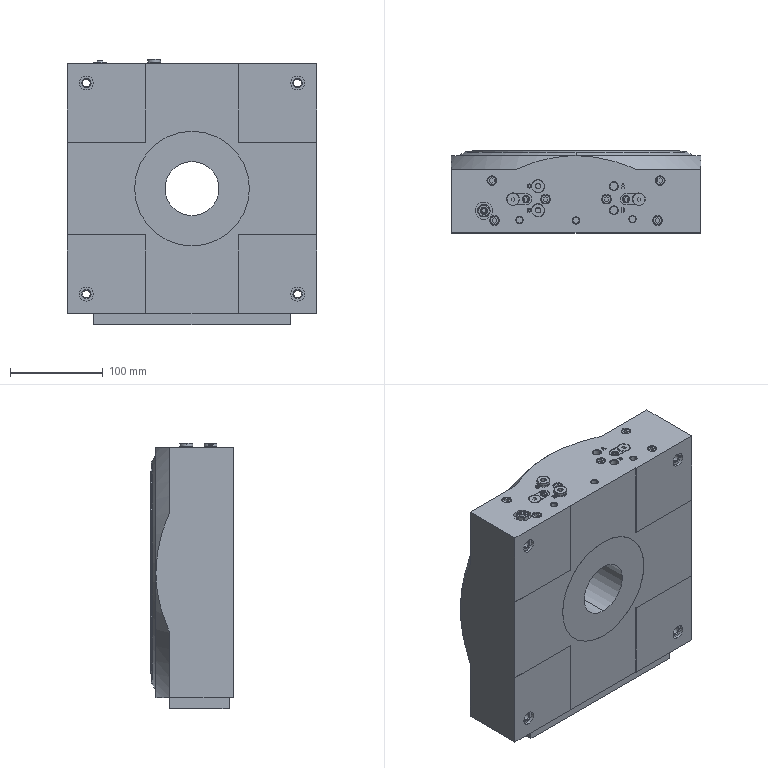Part | STEP file | 163302 DNC-32-200-P-A-V5---(asm_200)(index)_5 | 4 solids | 706 faces | box 270 x 89 x 286.6 mm | volume 5960531 mm3 | plane 390 | cylinder 165 | cone 135 | spline 16 | commonest cylinder face diameters 12 x13 4.134 x12 6.647 x12 10 x12 10.5 x12 14 x11